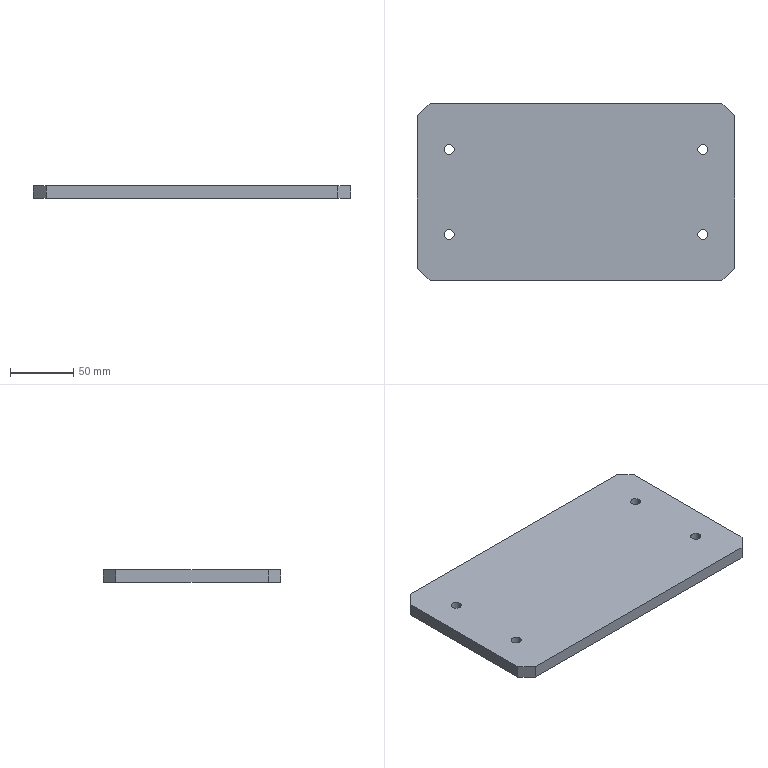Part | SolidWorks | features Cut 2, ICE 2, Extrusion 1 | 1 solid | 27 faces | box 250 x 140 x 10 mm | volume 345235 mm3 | cylinder 14 | plane 13 | commonest cylinder face diameters 8 x14
STEP:
#1=CARTESIAN_POINT('',(96.,-33.5,0.));
#2=VERTEX_POINT('',#1);
#3=CARTESIAN_POINT('',(104.,-33.5,0.));
#4=VERTEX_POINT('',#3);
#5=CARTESIAN_POINT('',(100.,-33.5,0.));
#6=DIRECTION('',(0.,0.,1.));
#7=DIRECTION('',(-1.,0.,0.));
#8=AXIS2_PLACEMENT_3D('',#5,#6,#7);
#9=CIRCLE('',#8,4.);
#10=EDGE_CURVE('',#2,#4,#9,.T.);
#11=ORIENTED_EDGE('',*,*,#10,.F.);
#12=CARTESIAN_POINT('',(96.,-33.5,10.));
#13=VERTEX_POINT('',#12);
#14=CARTESIAN_POINT('',(96.,-33.5,-11.314));
#15=DIRECTION('',(0.,0.,1.));
#16=VECTOR('',#15,1000.);
#17=LINE('',#14,#16);
#18=EDGE_CURVE('',#2,#13,#17,.T.);
#19=ORIENTED_EDGE('',*,*,#18,.T.);
#20=CARTESIAN_POINT('',(104.,-33.5,10.));
#21=VERTEX_POINT('',#20);
#22=CARTESIAN_POINT('',(100.,-33.5,10.));
#23=DIRECTION('',(0.,0.,1.));
#24=DIRECTION('',(-1.,0.,0.));
#25=AXIS2_PLACEMENT_3D('',#22,#23,#24);
#26=CIRCLE('',#25,4.);
#27=EDGE_CURVE('',#13,#21,#26,.T.);
#28=ORIENTED_EDGE('',*,*,#27,.T.);
#29=CARTESIAN_POINT('',(104.,-33.5,-11.314));
#30=DIRECTION('',(0.,0.,1.));
#31=VECTOR('',#30,1000.);
#32=LINE('',#29,#31);
#33=EDGE_CURVE('',#4,#21,#32,.T.);
#34=ORIENTED_EDGE('',*,*,#33,.F.);
#35=EDGE_LOOP('',(#11,#19,#28,#34));
#36=FACE_OUTER_BOUND('',#35,.T.);
#37=CARTESIAN_POINT('',(100.,-33.5,-11.314));
#38=DIRECTION('',(0.,0.,1.));
#39=DIRECTION('',(1.,0.,0.));
#40=AXIS2_PLACEMENT_3D('',#37,#38,#39);
#41=CYLINDRICAL_SURFACE('',#40,4.);
#42=ADVANCED_FACE('',(#36),#41,.F.);
#43=CARTESIAN_POINT('',(-104.,-33.5,0.));
#44=VERTEX_POINT('',#43);
#45=CARTESIAN_POINT('',(-96.,-33.5,0.));
#46=VERTEX_POINT('',#45);
#47=CARTESIAN_POINT('',(-100.,-33.5,0.));
#48=DIRECTION('',(0.,0.,1.));
#49=DIRECTION('',(-1.,0.,0.));
#50=AXIS2_PLACEMENT_3D('',#47,#48,#49);
#51=CIRCLE('',#50,4.);
#52=EDGE_CURVE('',#44,#46,#51,.T.);
#53=ORIENTED_EDGE('',*,*,#52,.F.);
#54=CARTESIAN_POINT('',(-104.,-33.5,10.));
#55=VERTEX_POINT('',#54);
#56=CARTESIAN_POINT('',(-104.,-33.5,-11.314));
#57=DIRECTION('',(0.,0.,1.));
#58=VECTOR('',#57,1000.);
#59=LINE('',#56,#58);
#60=EDGE_CURVE('',#44,#55,#59,.T.);
#61=ORIENTED_EDGE('',*,*,#60,.T.);
#62=CARTESIAN_POINT('',(-96.,-33.5,10.));
#63=VERTEX_POINT('',#62);
#64=CARTESIAN_POINT('',(-100.,-33.5,10.));
#65=DIRECTION('',(0.,0.,1.));
#66=DIRECTION('',(1.,0.,0.));
#67=AXIS2_PLACEMENT_3D('',#64,#65,#66);
#68=CIRCLE('',#67,4.);
#69=EDGE_CURVE('',#55,#63,#68,.T.);
#70=ORIENTED_EDGE('',*,*,#69,.T.);
#71=CARTESIAN_POINT('',(-96.,-33.5,-11.314));
#72=DIRECTION('',(0.,0.,1.));
#73=VECTOR('',#72,1000.);
#74=LINE('',#71,#73);
#75=EDGE_CURVE('',#46,#63,#74,.T.);
#76=ORIENTED_EDGE('',*,*,#75,.F.);
#77=EDGE_LOOP('',(#53,#61,#70,#76));
#78=FACE_OUTER_BOUND('',#77,.T.);
#79=CARTESIAN_POINT('',(-100.,-33.5,-11.314));
#80=DIRECTION('',(0.,0.,1.));
#81=DIRECTION('',(1.,0.,0.));
#82=AXIS2_PLACEMENT_3D('',#79,#80,#81);
#83=CYLINDRICAL_SURFACE('',#82,4.);
#84=ADVANCED_FACE('',(#78),#83,.F.);
#85=CARTESIAN_POINT('',(-104.,33.5,0.));
#86=VERTEX_POINT('',#85);
#87=CARTESIAN_POINT('',(-96.,33.5,0.));
#88=VERTEX_POINT('',#87);
#89=CARTESIAN_POINT('',(-100.,33.5,0.));
#90=DIRECTION('',(0.,0.,1.));
#91=DIRECTION('',(-1.,0.,0.));
#92=AXIS2_PLACEMENT_3D('',#89,#90,#91);
#93=CIRCLE('',#92,4.);
#94=EDGE_CURVE('',#86,#88,#93,.T.);
#95=ORIENTED_EDGE('',*,*,#94,.F.);
#96=CARTESIAN_POINT('',(-104.,33.5,10.));
#97=VERTEX_POINT('',#96);
#98=CARTESIAN_POINT('',(-104.,33.5,-11.314));
#99=DIRECTION('',(0.,0.,1.));
#100=VECTOR('',#99,1000.);
#101=LINE('',#98,#100);
#102=EDGE_CURVE('',#86,#97,#101,.T.);
#103=ORIENTED_EDGE('',*,*,#102,.T.);
#104=CARTESIAN_POINT('',(-96.,33.5,10.));
#105=VERTEX_POINT('',#104);
#106=CARTESIAN_POINT('',(-100.,33.5,10.));
#107=DIRECTION('',(0.,0.,1.));
#108=DIRECTION('',(-1.,0.,0.));
#109=AXIS2_PLACEMENT_3D('',#106,#107,#108);
#110=CIRCLE('',#109,4.);
#111=EDGE_CURVE('',#97,#105,#110,.T.);
#112=ORIENTED_EDGE('',*,*,#111,.T.);
#113=CARTESIAN_POINT('',(-96.,33.5,-11.314));
#114=DIRECTION('',(0.,0.,1.));
#115=VECTOR('',#114,1000.);
#116=LINE('',#113,#115);
#117=EDGE_CURVE('',#88,#105,#116,.T.);
#118=ORIENTED_EDGE('',*,*,#117,.F.);
#119=EDGE_LOOP('',(#95,#103,#112,#118));
#120=FACE_OUTER_BOUND('',#119,.T.);
#121=CARTESIAN_POINT('',(-100.,33.5,-11.314));
#122=DIRECTION('',(0.,0.,1.));
#123=DIRECTION('',(1.,0.,0.));
#124=AXIS2_PLACEMENT_3D('',#121,#122,#123);
#125=CYLINDRICAL_SURFACE('',#124,4.);
#126=ADVANCED_FACE('',(#120),#125,.F.);
#127=CARTESIAN_POINT('',(96.,33.5,0.));
#128=VERTEX_POINT('',#127);
#129=CARTESIAN_POINT('',(104.,33.5,0.));
#130=VERTEX_POINT('',#129);
#131=CARTESIAN_POINT('',(100.,33.5,0.));
#132=DIRECTION('',(0.,0.,1.));
#133=DIRECTION('',(-1.,0.,0.));
#134=AXIS2_PLACEMENT_3D('',#131,#132,#133);
#135=CIRCLE('',#134,4.);
#136=EDGE_CURVE('',#128,#130,#135,.T.);
#137=ORIENTED_EDGE('',*,*,#136,.F.);
#138=CARTESIAN_POINT('',(96.,33.5,10.));
#139=VERTEX_POINT('',#138);
#140=CARTESIAN_POINT('',(96.,33.5,-11.314));
#141=DIRECTION('',(0.,0.,1.));
#142=VECTOR('',#141,1000.);
#143=LINE('',#140,#142);
#144=EDGE_CURVE('',#128,#139,#143,.T.);
#145=ORIENTED_EDGE('',*,*,#144,.T.);
#146=CARTESIAN_POINT('',(104.,33.5,10.));
#147=VERTEX_POINT('',#146);
#148=CARTESIAN_POINT('',(100.,33.5,10.));
#149=DIRECTION('',(0.,0.,1.));
#150=DIRECTION('',(1.,0.,0.));
#151=AXIS2_PLACEMENT_3D('',#148,#149,#150);
#152=CIRCLE('',#151,4.);
#153=EDGE_CURVE('',#139,#147,#152,.T.);
#154=ORIENTED_EDGE('',*,*,#153,.T.);
#155=CARTESIAN_POINT('',(104.,33.5,-11.314));
#156=DIRECTION('',(0.,0.,1.));
#157=VECTOR('',#156,1000.);
#158=LINE('',#155,#157);
#159=EDGE_CURVE('',#130,#147,#158,.T.);
#160=ORIENTED_EDGE('',*,*,#159,.F.);
#161=EDGE_LOOP('',(#137,#145,#154,#160));
#162=FACE_OUTER_BOUND('',#161,.T.);
#163=CARTESIAN_POINT('',(100.,33.5,-11.314));
#164=DIRECTION('',(0.,0.,1.));
#165=DIRECTION('',(1.,0.,0.));
#166=AXIS2_PLACEMENT_3D('',#163,#164,#165);
#167=CYLINDRICAL_SURFACE('',#166,4.);
#168=ADVANCED_FACE('',(#162),#167,.F.);
#169=CARTESIAN_POINT('',(54.,-64.1,5.));
#170=VERTEX_POINT('',#169);
#171=CARTESIAN_POINT('',(46.,-64.1,5.));
#172=VERTEX_POINT('',#171);
#173=CARTESIAN_POINT('',(50.,-64.1,5.));
#174=DIRECTION('',(0.,0.,-1.));
#175=DIRECTION('',(-1.,0.,0.));
#176=AXIS2_PLACEMENT_3D('',#173,#174,#175);
#177=CIRCLE('',#176,4.);
#178=EDGE_CURVE('',#170,#172,#177,.T.);
#179=ORIENTED_EDGE('',*,*,#178,.F.);
#180=CARTESIAN_POINT('',(54.,-64.1,0.));
#181=VERTEX_POINT('',#180);
#182=CARTESIAN_POINT('',(54.,-64.1,5.));
#183=DIRECTION('',(0.,0.,-1.));
#184=VECTOR('',#183,1000.);
#185=LINE('',#182,#184);
#186=EDGE_CURVE('',#170,#181,#185,.T.);
#187=ORIENTED_EDGE('',*,*,#186,.T.);
#188=CARTESIAN_POINT('',(46.,-64.1,0.));
#189=VERTEX_POINT('',#188);
#190=CARTESIAN_POINT('',(50.,-64.1,0.));
#191=DIRECTION('',(0.,0.,-1.));
#192=DIRECTION('',(-1.,0.,0.));
#193=AXIS2_PLACEMENT_3D('',#190,#191,#192);
#194=CIRCLE('',#193,4.);
#195=EDGE_CURVE('',#181,#189,#194,.T.);
#196=ORIENTED_EDGE('',*,*,#195,.T.);
#197=CARTESIAN_POINT('',(46.,-64.1,5.));
#198=DIRECTION('',(0.,0.,-1.));
#199=VECTOR('',#198,1000.);
#200=LINE('',#197,#199);
#201=EDGE_CURVE('',#172,#189,#200,.T.);
#202=ORIENTED_EDGE('',*,*,#201,.F.);
#203=EDGE_LOOP('',(#179,#187,#196,#202));
#204=FACE_OUTER_BOUND('',#203,.T.);
#205=CARTESIAN_POINT('',(50.,-64.1,5.));
#206=DIRECTION('',(0.,0.,-1.));
#207=DIRECTION('',(-1.,0.,0.));
#208=AXIS2_PLACEMENT_3D('',#205,#206,#207);
#209=CYLINDRICAL_SURFACE('',#208,4.);
#210=ADVANCED_FACE('',(#204),#209,.F.);
#211=CARTESIAN_POINT('',(-46.,-64.1,5.));
#212=VERTEX_POINT('',#211);
#213=CARTESIAN_POINT('',(-54.,-64.1,5.));
#214=VERTEX_POINT('',#213);
#215=CARTESIAN_POINT('',(-50.,-64.1,5.));
#216=DIRECTION('',(0.,0.,-1.));
#217=DIRECTION('',(1.,0.,0.));
#218=AXIS2_PLACEMENT_3D('',#215,#216,#217);
#219=CIRCLE('',#218,4.);
#220=EDGE_CURVE('',#212,#214,#219,.T.);
#221=ORIENTED_EDGE('',*,*,#220,.F.);
#222=CARTESIAN_POINT('',(-46.,-64.1,0.));
#223=VERTEX_POINT('',#222);
#224=CARTESIAN_POINT('',(-46.,-64.1,5.));
#225=DIRECTION('',(0.,0.,-1.));
#226=VECTOR('',#225,1000.);
#227=LINE('',#224,#226);
#228=EDGE_CURVE('',#212,#223,#227,.T.);
#229=ORIENTED_EDGE('',*,*,#228,.T.);
#230=CARTESIAN_POINT('',(-54.,-64.1,0.));
#231=VERTEX_POINT('',#230);
#232=CARTESIAN_POINT('',(-50.,-64.1,0.));
#233=DIRECTION('',(0.,0.,-1.));
#234=DIRECTION('',(1.,0.,0.));
#235=AXIS2_PLACEMENT_3D('',#232,#233,#234);
#236=CIRCLE('',#235,4.);
#237=EDGE_CURVE('',#223,#231,#236,.T.);
#238=ORIENTED_EDGE('',*,*,#237,.T.);
#239=CARTESIAN_POINT('',(-54.,-64.1,5.));
#240=DIRECTION('',(0.,0.,-1.));
#241=VECTOR('',#240,1000.);
#242=LINE('',#239,#241);
#243=EDGE_CURVE('',#214,#231,#242,.T.);
#244=ORIENTED_EDGE('',*,*,#243,.F.);
#245=EDGE_LOOP('',(#221,#229,#238,#244));
#246=FACE_OUTER_BOUND('',#245,.T.);
#247=CARTESIAN_POINT('',(-50.,-64.1,5.));
#248=DIRECTION('',(0.,0.,-1.));
#249=DIRECTION('',(-1.,0.,0.));
#250=AXIS2_PLACEMENT_3D('',#247,#248,#249);
#251=CYLINDRICAL_SURFACE('',#250,4.);
#252=ADVANCED_FACE('',(#246),#251,.F.);
#253=CARTESIAN_POINT('',(83.1,0.,5.));
#254=VERTEX_POINT('',#253);
#255=CARTESIAN_POINT('',(75.1,0.,5.));
#256=VERTEX_POINT('',#255);
#257=CARTESIAN_POINT('',(79.1,0.,5.));
#258=DIRECTION('',(0.,0.,-1.));
#259=DIRECTION('',(1.,0.,0.));
#260=AXIS2_PLACEMENT_3D('',#257,#258,#259);
#261=CIRCLE('',#260,4.);
#262=EDGE_CURVE('',#254,#256,#261,.T.);
#263=ORIENTED_EDGE('',*,*,#262,.F.);
#264=CARTESIAN_POINT('',(83.1,0.,0.));
#265=VERTEX_POINT('',#264);
#266=CARTESIAN_POINT('',(83.1,0.,5.));
#267=DIRECTION('',(0.,0.,-1.));
#268=VECTOR('',#267,1000.);
#269=LINE('',#266,#268);
#270=EDGE_CURVE('',#254,#265,#269,.T.);
#271=ORIENTED_EDGE('',*,*,#270,.T.);
#272=CARTESIAN_POINT('',(75.1,0.,0.));
#273=VERTEX_POINT('',#272);
#274=CARTESIAN_POINT('',(79.1,0.,0.));
#275=DIRECTION('',(0.,0.,-1.));
#276=DIRECTION('',(1.,0.,0.));
#277=AXIS2_PLACEMENT_3D('',#274,#275,#276);
#278=CIRCLE('',#277,4.);
#279=EDGE_CURVE('',#265,#273,#278,.T.);
#280=ORIENTED_EDGE('',*,*,#279,.T.);
#281=CARTESIAN_POINT('',(75.1,0.,5.));
#282=DIRECTION('',(0.,0.,-1.));
#283=VECTOR('',#282,1000.);
#284=LINE('',#281,#283);
#285=EDGE_CURVE('',#256,#273,#284,.T.);
#286=ORIENTED_EDGE('',*,*,#285,.F.);
#287=EDGE_LOOP('',(#263,#271,#280,#286));
#288=FACE_OUTER_BOUND('',#287,.T.);
#289=CARTESIAN_POINT('',(79.1,0.,5.));
#290=DIRECTION('',(0.,0.,-1.));
#291=DIRECTION('',(-1.,0.,0.));
#292=AXIS2_PLACEMENT_3D('',#289,#290,#291);
#293=CYLINDRICAL_SURFACE('',#292,4.);
#294=ADVANCED_FACE('',(#288),#293,.F.);
#295=CARTESIAN_POINT('',(115.,70.,0.));
#296=VERTEX_POINT('',#295);
#297=CARTESIAN_POINT('',(-115.,70.,0.));
#298=VERTEX_POINT('',#297);
#299=CARTESIAN_POINT('',(115.,70.,0.));
#300=DIRECTION('',(-1.,0.,0.));
#301=VECTOR('',#300,1000.);
#302=LINE('',#299,#301);
#303=EDGE_CURVE('',#296,#298,#302,.T.);
#304=ORIENTED_EDGE('',*,*,#303,.T.);
#305=CARTESIAN_POINT('',(-115.,70.,10.));
#306=VERTEX_POINT('',#305);
#307=CARTESIAN_POINT('',(-115.,70.,10.));
#308=DIRECTION('',(0.,0.,-1.));
#309=VECTOR('',#308,1000.);
#310=LINE('',#307,#309);
#311=EDGE_CURVE('',#306,#298,#310,.T.);
#312=ORIENTED_EDGE('',*,*,#311,.F.);
#313=CARTESIAN_POINT('',(115.,70.,10.));
#314=VERTEX_POINT('',#313);
#315=CARTESIAN_POINT('',(115.,70.,10.));
#316=DIRECTION('',(-1.,0.,0.));
#317=VECTOR('',#316,1000.);
#318=LINE('',#315,#317);
#319=EDGE_CURVE('',#314,#306,#318,.T.);
#320=ORIENTED_EDGE('',*,*,#319,.F.);
#321=CARTESIAN_POINT('',(115.,70.,10.));
#322=DIRECTION('',(0.,0.,-1.));
#323=VECTOR('',#322,1000.);
#324=LINE('',#321,#323);
#325=EDGE_CURVE('',#314,#296,#324,.T.);
#326=ORIENTED_EDGE('',*,*,#325,.T.);
#327=EDGE_LOOP('',(#304,#312,#320,#326));
#328=FACE_OUTER_BOUND('',#327,.T.);
#329=CARTESIAN_POINT('',(115.,70.,10.));
#330=DIRECTION('',(0.,-1.,0.));
#331=DIRECTION('',(1.,0.,0.));
#332=AXIS2_PLACEMENT_3D('',#329,#330,#331);
#333=PLANE('',#332);
#334=ADVANCED_FACE('',(#328),#333,.F.);
#335=CARTESIAN_POINT('',(-125.,60.,0.));
#336=VERTEX_POINT('',#335);
#337=CARTESIAN_POINT('',(-115.,70.,0.));
#338=DIRECTION('',(-0.7071,-0.7071,0.));
#339=VECTOR('',#338,1000.);
#340=LINE('',#337,#339);
#341=EDGE_CURVE('',#298,#336,#340,.T.);
#342=ORIENTED_EDGE('',*,*,#341,.T.);
#343=CARTESIAN_POINT('',(-125.,60.,10.));
#344=VERTEX_POINT('',#343);
#345=CARTESIAN_POINT('',(-125.,60.,10.));
#346=DIRECTION('',(0.,0.,-1.));
#347=VECTOR('',#346,1000.);
#348=LINE('',#345,#347);
#349=EDGE_CURVE('',#344,#336,#348,.T.);
#350=ORIENTED_EDGE('',*,*,#349,.F.);
#351=CARTESIAN_POINT('',(-115.,70.,10.));
#352=DIRECTION('',(-0.7071,-0.7071,0.));
#353=VECTOR('',#352,1000.);
#354=LINE('',#351,#353);
#355=EDGE_CURVE('',#306,#344,#354,.T.);
#356=ORIENTED_EDGE('',*,*,#355,.F.);
#357=ORIENTED_EDGE('',*,*,#311,.T.);
#358=EDGE_LOOP('',(#342,#350,#356,#357));
#359=FACE_OUTER_BOUND('',#358,.T.);
#360=CARTESIAN_POINT('',(-115.,70.,10.));
#361=DIRECTION('',(0.7071,-0.7071,0.));
#362=DIRECTION('',(0.7071,0.7071,0.));
#363=AXIS2_PLACEMENT_3D('',#360,#361,#362);
#364=PLANE('',#363);
#365=ADVANCED_FACE('',(#359),#364,.F.);
#366=CARTESIAN_POINT('',(-125.,-60.,0.));
#367=VERTEX_POINT('',#366);
#368=CARTESIAN_POINT('',(-125.,-60.,0.));
#369=DIRECTION('',(0.,-1.,0.));
#370=VECTOR('',#369,1000.);
#371=LINE('',#368,#370);
#372=EDGE_CURVE('',#336,#367,#371,.T.);
#373=ORIENTED_EDGE('',*,*,#372,.T.);
#374=CARTESIAN_POINT('',(-125.,-60.,10.));
#375=VERTEX_POINT('',#374);
#376=CARTESIAN_POINT('',(-125.,-60.,10.));
#377=DIRECTION('',(0.,0.,-1.));
#378=VECTOR('',#377,1000.);
#379=LINE('',#376,#378);
#380=EDGE_CURVE('',#375,#367,#379,.T.);
#381=ORIENTED_EDGE('',*,*,#380,.F.);
#382=CARTESIAN_POINT('',(-125.,-60.,10.));
#383=DIRECTION('',(0.,-1.,0.));
#384=VECTOR('',#383,1000.);
#385=LINE('',#382,#384);
#386=EDGE_CURVE('',#344,#375,#385,.T.);
#387=ORIENTED_EDGE('',*,*,#386,.F.);
#388=ORIENTED_EDGE('',*,*,#349,.T.);
#389=EDGE_LOOP('',(#373,#381,#387,#388));
#390=FACE_OUTER_BOUND('',#389,.T.);
#391=CARTESIAN_POINT('',(-125.,-60.,10.));
#392=DIRECTION('',(1.,0.,0.));
#393=DIRECTION('',(0.,0.,-1.));
#394=AXIS2_PLACEMENT_3D('',#391,#392,#393);
#395=PLANE('',#394);
#396=ADVANCED_FACE('',(#390),#395,.F.);
#397=CARTESIAN_POINT('',(-115.,-70.,0.));
#398=VERTEX_POINT('',#397);
#399=CARTESIAN_POINT('',(-115.,-70.,0.));
#400=DIRECTION('',(0.7071,-0.7071,0.));
#401=VECTOR('',#400,1000.);
#402=LINE('',#399,#401);
#403=EDGE_CURVE('',#367,#398,#402,.T.);
#404=ORIENTED_EDGE('',*,*,#403,.T.);
#405=CARTESIAN_POINT('',(-115.,-70.,10.));
#406=VERTEX_POINT('',#405);
#407=CARTESIAN_POINT('',(-115.,-70.,10.));
#408=DIRECTION('',(0.,0.,-1.));
#409=VECTOR('',#408,1000.);
#410=LINE('',#407,#409);
#411=EDGE_CURVE('',#406,#398,#410,.T.);
#412=ORIENTED_EDGE('',*,*,#411,.F.);
#413=CARTESIAN_POINT('',(-115.,-70.,10.));
#414=DIRECTION('',(0.7071,-0.7071,0.));
#415=VECTOR('',#414,1000.);
#416=LINE('',#413,#415);
#417=EDGE_CURVE('',#375,#406,#416,.T.);
#418=ORIENTED_EDGE('',*,*,#417,.F.);
#419=ORIENTED_EDGE('',*,*,#380,.T.);
#420=EDGE_LOOP('',(#404,#412,#418,#419));
#421=FACE_OUTER_BOUND('',#420,.T.);
#422=CARTESIAN_POINT('',(-115.,-70.,10.));
#423=DIRECTION('',(0.7071,0.7071,0.));
#424=DIRECTION('',(-0.7071,0.7071,0.));
#425=AXIS2_PLACEMENT_3D('',#422,#423,#424);
#426=PLANE('',#425);
#427=ADVANCED_FACE('',(#421),#426,.F.);
#428=CARTESIAN_POINT('',(115.,-70.,0.));
#429=VERTEX_POINT('',#428);
#430=CARTESIAN_POINT('',(115.,-70.,0.));
#431=DIRECTION('',(1.,0.,0.));
#432=VECTOR('',#431,1000.);
#433=LINE('',#430,#432);
#434=EDGE_CURVE('',#398,#429,#433,.T.);
#435=ORIENTED_EDGE('',*,*,#434,.T.);
#436=CARTESIAN_POINT('',(115.,-70.,10.));
#437=VERTEX_POINT('',#436);
#438=CARTESIAN_POINT('',(115.,-70.,10.));
#439=DIRECTION('',(0.,0.,-1.));
#440=VECTOR('',#439,1000.);
#441=LINE('',#438,#440);
#442=EDGE_CURVE('',#437,#429,#441,.T.);
#443=ORIENTED_EDGE('',*,*,#442,.F.);
#444=CARTESIAN_POINT('',(115.,-70.,10.));
#445=DIRECTION('',(1.,0.,0.));
#446=VECTOR('',#445,1000.);
#447=LINE('',#444,#446);
#448=EDGE_CURVE('',#406,#437,#447,.T.);
#449=ORIENTED_EDGE('',*,*,#448,.F.);
#450=ORIENTED_EDGE('',*,*,#411,.T.);
#451=EDGE_LOOP('',(#435,#443,#449,#450));
#452=FACE_OUTER_BOUND('',#451,.T.);
#453=CARTESIAN_POINT('',(115.,-70.,10.));
#454=DIRECTION('',(0.,1.,0.));
#455=DIRECTION('',(-1.,0.,0.));
#456=AXIS2_PLACEMENT_3D('',#453,#454,#455);
#457=PLANE('',#456);
#458=ADVANCED_FACE('',(#452),#457,.F.);
#459=CARTESIAN_POINT('',(125.,-60.,0.));
#460=VERTEX_POINT('',#459);
#461=CARTESIAN_POINT('',(115.,-70.,0.));
#462=DIRECTION('',(0.7071,0.7071,0.));
#463=VECTOR('',#462,1000.);
#464=LINE('',#461,#463);
#465=EDGE_CURVE('',#429,#460,#464,.T.);
#466=ORIENTED_EDGE('',*,*,#465,.T.);
#467=CARTESIAN_POINT('',(125.,-60.,10.));
#468=VERTEX_POINT('',#467);
#469=CARTESIAN_POINT('',(125.,-60.,10.));
#470=DIRECTION('',(0.,0.,-1.));
#471=VECTOR('',#470,1000.);
#472=LINE('',#469,#471);
#473=EDGE_CURVE('',#468,#460,#472,.T.);
#474=ORIENTED_EDGE('',*,*,#473,.F.);
#475=CARTESIAN_POINT('',(115.,-70.,10.));
#476=DIRECTION('',(0.7071,0.7071,0.));
#477=VECTOR('',#476,1000.);
#478=LINE('',#475,#477);
#479=EDGE_CURVE('',#437,#468,#478,.T.);
#480=ORIENTED_EDGE('',*,*,#479,.F.);
#481=ORIENTED_EDGE('',*,*,#442,.T.);
#482=EDGE_LOOP('',(#466,#474,#480,#481));
#483=FACE_OUTER_BOUND('',#482,.T.);
#484=CARTESIAN_POINT('',(115.,-70.,10.));
#485=DIRECTION('',(-0.7071,0.7071,0.));
#486=DIRECTION('',(-0.7071,-0.7071,0.));
#487=AXIS2_PLACEMENT_3D('',#484,#485,#486);
#488=PLANE('',#487);
#489=ADVANCED_FACE('',(#483),#488,.F.);
#490=CARTESIAN_POINT('',(125.,60.,0.));
#491=VERTEX_POINT('',#490);
#492=CARTESIAN_POINT('',(125.,-60.,0.));
#493=DIRECTION('',(0.,1.,0.));
#494=VECTOR('',#493,1000.);
#495=LINE('',#492,#494);
#496=EDGE_CURVE('',#460,#491,#495,.T.);
#497=ORIENTED_EDGE('',*,*,#496,.T.);
#498=CARTESIAN_POINT('',(125.,60.,10.));
#499=VERTEX_POINT('',#498);
#500=CARTESIAN_POINT('',(125.,60.,10.));
#501=DIRECTION('',(0.,0.,-1.));
#502=VECTOR('',#501,1000.);
#503=LINE('',#500,#502);
#504=EDGE_CURVE('',#499,#491,#503,.T.);
#505=ORIENTED_EDGE('',*,*,#504,.F.);
#506=CARTESIAN_POINT('',(125.,-60.,10.));
#507=DIRECTION('',(0.,1.,0.));
#508=VECTOR('',#507,1000.);
#509=LINE('',#506,#508);
#510=EDGE_CURVE('',#468,#499,#509,.T.);
#511=ORIENTED_EDGE('',*,*,#510,.F.);
#512=ORIENTED_EDGE('',*,*,#473,.T.);
#513=EDGE_LOOP('',(#497,#505,#511,#512));
#514=FACE_OUTER_BOUND('',#513,.T.);
#515=CARTESIAN_POINT('',(125.,-60.,10.));
#516=DIRECTION('',(-1.,0.,0.));
#517=DIRECTION('',(0.,0.,1.));
#518=AXIS2_PLACEMENT_3D('',#515,#516,#517);
#519=PLANE('',#518);
#520=ADVANCED_FACE('',(#514),#519,.F.);
#521=CARTESIAN_POINT('',(125.,60.,0.));
#522=DIRECTION('',(-0.7071,0.7071,0.));
#523=VECTOR('',#522,1000.);
#524=LINE('',#521,#523);
#525=EDGE_CURVE('',#491,#296,#524,.T.);
#526=ORIENTED_EDGE('',*,*,#525,.T.);
#527=ORIENTED_EDGE('',*,*,#325,.F.);
#528=CARTESIAN_POINT('',(125.,60.,10.));
#529=DIRECTION('',(-0.7071,0.7071,0.));
#530=VECTOR('',#529,1000.);
#531=LINE('',#528,#530);
#532=EDGE_CURVE('',#499,#314,#531,.T.);
#533=ORIENTED_EDGE('',*,*,#532,.F.);
#534=ORIENTED_EDGE('',*,*,#504,.T.);
#535=EDGE_LOOP('',(#526,#527,#533,#534));
#536=FACE_OUTER_BOUND('',#535,.T.);
#537=CARTESIAN_POINT('',(125.,60.,10.));
#538=DIRECTION('',(-0.7071,-0.7071,0.));
#539=DIRECTION('',(0.7071,-0.7071,0.));
#540=AXIS2_PLACEMENT_3D('',#537,#538,#539);
#541=PLANE('',#540);
#542=ADVANCED_FACE('',(#536),#541,.F.);
#543=CARTESIAN_POINT('',(100.,-33.5,10.));
#544=DIRECTION('',(0.,0.,1.));
#545=DIRECTION('',(-1.,0.,0.));
#546=AXIS2_PLACEMENT_3D('',#543,#544,#545);
#547=CIRCLE('',#546,4.);
#548=EDGE_CURVE('',#21,#13,#547,.T.);
#549=ORIENTED_EDGE('',*,*,#548,.F.);
#550=ORIENTED_EDGE('',*,*,#27,.F.);
#551=EDGE_LOOP('',(#549,#550));
#552=FACE_BOUND('',#551,.T.);
#553=CARTESIAN_POINT('',(-100.,-33.5,10.));
#554=DIRECTION('',(0.,0.,1.));
#555=DIRECTION('',(1.,0.,0.));
#556=AXIS2_PLACEMENT_3D('',#553,#554,#555);
#557=CIRCLE('',#556,4.);
#558=EDGE_CURVE('',#63,#55,#557,.T.);
#559=ORIENTED_EDGE('',*,*,#558,.F.);
#560=ORIENTED_EDGE('',*,*,#69,.F.);
#561=EDGE_LOOP('',(#559,#560));
#562=FACE_BOUND('',#561,.T.);
#563=CARTESIAN_POINT('',(-100.,33.5,10.));
#564=DIRECTION('',(0.,0.,1.));
#565=DIRECTION('',(-1.,0.,0.));
#566=AXIS2_PLACEMENT_3D('',#563,#564,#565);
#567=CIRCLE('',#566,4.);
#568=EDGE_CURVE('',#105,#97,#567,.T.);
#569=ORIENTED_EDGE('',*,*,#568,.F.);
#570=ORIENTED_EDGE('',*,*,#111,.F.);
#571=EDGE_LOOP('',(#569,#570));
#572=FACE_BOUND('',#571,.T.);
#573=CARTESIAN_POINT('',(100.,33.5,10.));
#574=DIRECTION('',(0.,0.,1.));
#575=DIRECTION('',(1.,0.,0.));
#576=AXIS2_PLACEMENT_3D('',#573,#574,#575);
#577=CIRCLE('',#576,4.);
#578=EDGE_CURVE('',#147,#139,#577,.T.);
#579=ORIENTED_EDGE('',*,*,#578,.F.);
#580=ORIENTED_EDGE('',*,*,#153,.F.);
#581=EDGE_LOOP('',(#579,#580));
#582=FACE_BOUND('',#581,.T.);
#583=ORIENTED_EDGE('',*,*,#319,.T.);
#584=ORIENTED_EDGE('',*,*,#355,.T.);
#585=ORIENTED_EDGE('',*,*,#386,.T.);
#586=ORIENTED_EDGE('',*,*,#417,.T.);
#587=ORIENTED_EDGE('',*,*,#448,.T.);
#588=ORIENTED_EDGE('',*,*,#479,.T.);
#589=ORIENTED_EDGE('',*,*,#510,.T.);
#590=ORIENTED_EDGE('',*,*,#532,.T.);
#591=EDGE_LOOP('',(#583,#584,#585,#586,#587,#588,#589,#590));
#592=FACE_OUTER_BOUND('',#591,.T.);
#593=CARTESIAN_POINT('',(0.,0.,10.));
#594=DIRECTION('',(0.,0.,-1.));
#595=DIRECTION('',(-1.,0.,0.));
#596=AXIS2_PLACEMENT_3D('',#593,#594,#595);
#597=PLANE('',#596);
#598=ADVANCED_FACE('',(#552,#562,#572,#582,#592),#597,.F.);
#599=CARTESIAN_POINT('',(100.,-33.5,0.));
#600=DIRECTION('',(0.,0.,1.));
#601=DIRECTION('',(-1.,0.,0.));
#602=AXIS2_PLACEMENT_3D('',#599,#600,#601);
#603=CIRCLE('',#602,4.);
#604=EDGE_CURVE('',#4,#2,#603,.T.);
#605=ORIENTED_EDGE('',*,*,#604,.T.);
#606=ORIENTED_EDGE('',*,*,#10,.T.);
#607=EDGE_LOOP('',(#605,#606));
#608=FACE_BOUND('',#607,.T.);
#609=CARTESIAN_POINT('',(-100.,-33.5,0.));
#610=DIRECTION('',(0.,0.,1.));
#611=DIRECTION('',(-1.,0.,0.));
#612=AXIS2_PLACEMENT_3D('',#609,#610,#611);
#613=CIRCLE('',#612,4.);
#614=EDGE_CURVE('',#46,#44,#613,.T.);
#615=ORIENTED_EDGE('',*,*,#614,.T.);
#616=ORIENTED_EDGE('',*,*,#52,.T.);
#617=EDGE_LOOP('',(#615,#616));
#618=FACE_BOUND('',#617,.T.);
#619=CARTESIAN_POINT('',(-100.,33.5,0.));
#620=DIRECTION('',(0.,0.,1.));
#621=DIRECTION('',(-1.,0.,0.));
#622=AXIS2_PLACEMENT_3D('',#619,#620,#621);
#623=CIRCLE('',#622,4.);
#624=EDGE_CURVE('',#88,#86,#623,.T.);
#625=ORIENTED_EDGE('',*,*,#624,.T.);
#626=ORIENTED_EDGE('',*,*,#94,.T.);
#627=EDGE_LOOP('',(#625,#626));
#628=FACE_BOUND('',#627,.T.);
#629=CARTESIAN_POINT('',(100.,33.5,0.));
#630=DIRECTION('',(0.,0.,1.));
#631=DIRECTION('',(-1.,0.,0.));
#632=AXIS2_PLACEMENT_3D('',#629,#630,#631);
#633=CIRCLE('',#632,4.);
#634=EDGE_CURVE('',#130,#128,#633,.T.);
#635=ORIENTED_EDGE('',*,*,#634,.T.);
#636=ORIENTED_EDGE('',*,*,#136,.T.);
#637=EDGE_LOOP('',(#635,#636));
#638=FACE_BOUND('',#637,.T.);
#639=CARTESIAN_POINT('',(50.,-64.1,0.));
#640=DIRECTION('',(0.,0.,-1.));
#641=DIRECTION('',(-1.,0.,0.));
#642=AXIS2_PLACEMENT_3D('',#639,#640,#641);
#643=CIRCLE('',#642,4.);
#644=EDGE_CURVE('',#189,#181,#643,.T.);
#645=ORIENTED_EDGE('',*,*,#644,.F.);
#646=ORIENTED_EDGE('',*,*,#195,.F.);
#647=EDGE_LOOP('',(#645,#646));
#648=FACE_BOUND('',#647,.T.);
#649=CARTESIAN_POINT('',(-50.,-64.1,0.));
#650=DIRECTION('',(0.,0.,-1.));
#651=DIRECTION('',(1.,0.,0.));
#652=AXIS2_PLACEMENT_3D('',#649,#650,#651);
#653=CIRCLE('',#652,4.);
#654=EDGE_CURVE('',#231,#223,#653,.T.);
#655=ORIENTED_EDGE('',*,*,#654,.F.);
#656=ORIENTED_EDGE('',*,*,#237,.F.);
#657=EDGE_LOOP('',(#655,#656));
#658=FACE_BOUND('',#657,.T.);
#659=CARTESIAN_POINT('',(79.1,0.,0.));
#660=DIRECTION('',(0.,0.,-1.));
#661=DIRECTION('',(1.,0.,0.));
#662=AXIS2_PLACEMENT_3D('',#659,#660,#661);
#663=CIRCLE('',#662,4.);
#664=EDGE_CURVE('',#273,#265,#663,.T.);
#665=ORIENTED_EDGE('',*,*,#664,.F.);
#666=ORIENTED_EDGE('',*,*,#279,.F.);
#667=EDGE_LOOP('',(#665,#666));
#668=FACE_BOUND('',#667,.T.);
#669=ORIENTED_EDGE('',*,*,#303,.F.);
#670=ORIENTED_EDGE('',*,*,#525,.F.);
#671=ORIENTED_EDGE('',*,*,#496,.F.);
#672=ORIENTED_EDGE('',*,*,#465,.F.);
#673=ORIENTED_EDGE('',*,*,#434,.F.);
#674=ORIENTED_EDGE('',*,*,#403,.F.);
#675=ORIENTED_EDGE('',*,*,#372,.F.);
#676=ORIENTED_EDGE('',*,*,#341,.F.);
#677=EDGE_LOOP('',(#669,#670,#671,#672,#673,#674,#675,#676));
#678=FACE_OUTER_BOUND('',#677,.T.);
#679=CARTESIAN_POINT('',(0.,0.,0.));
#680=DIRECTION('',(0.,0.,-1.));
#681=DIRECTION('',(-1.,0.,0.));
#682=AXIS2_PLACEMENT_3D('',#679,#680,#681);
#683=PLANE('',#682);
#684=ADVANCED_FACE('',(#608,#618,#628,#638,#648,#658,#668,#678),#683,.T.);
#685=ORIENTED_EDGE('',*,*,#270,.F.);
#686=CARTESIAN_POINT('',(79.1,0.,5.));
#687=DIRECTION('',(0.,0.,-1.));
#688=DIRECTION('',(1.,0.,0.));
#689=AXIS2_PLACEMENT_3D('',#686,#687,#688);
#690=CIRCLE('',#689,4.);
#691=EDGE_CURVE('',#256,#254,#690,.T.);
#692=ORIENTED_EDGE('',*,*,#691,.F.);
#693=ORIENTED_EDGE('',*,*,#285,.T.);
#694=ORIENTED_EDGE('',*,*,#664,.T.);
#695=EDGE_LOOP('',(#685,#692,#693,#694));
#696=FACE_OUTER_BOUND('',#695,.T.);
#697=CARTESIAN_POINT('',(79.1,0.,5.));
#698=DIRECTION('',(0.,0.,-1.));
#699=DIRECTION('',(-1.,0.,0.));
#700=AXIS2_PLACEMENT_3D('',#697,#698,#699);
#701=CYLINDRICAL_SURFACE('',#700,4.);
#702=ADVANCED_FACE('',(#696),#701,.F.);
#703=ORIENTED_EDGE('',*,*,#691,.T.);
#704=ORIENTED_EDGE('',*,*,#262,.T.);
#705=EDGE_LOOP('',(#703,#704));
#706=FACE_OUTER_BOUND('',#705,.T.);
#707=CARTESIAN_POINT('',(79.1,0.,5.));
#708=DIRECTION('',(0.,0.,1.));
#709=DIRECTION('',(1.,0.,0.));
#710=AXIS2_PLACEMENT_3D('',#707,#708,#709);
#711=PLANE('',#710);
#712=ADVANCED_FACE('',(#706),#711,.F.);
#713=ORIENTED_EDGE('',*,*,#228,.F.);
#714=CARTESIAN_POINT('',(-50.,-64.1,5.));
#715=DIRECTION('',(0.,0.,-1.));
#716=DIRECTION('',(1.,0.,0.));
#717=AXIS2_PLACEMENT_3D('',#714,#715,#716);
#718=CIRCLE('',#717,4.);
#719=EDGE_CURVE('',#214,#212,#718,.T.);
#720=ORIENTED_EDGE('',*,*,#719,.F.);
#721=ORIENTED_EDGE('',*,*,#243,.T.);
#722=ORIENTED_EDGE('',*,*,#654,.T.);
#723=EDGE_LOOP('',(#713,#720,#721,#722));
#724=FACE_OUTER_BOUND('',#723,.T.);
#725=CARTESIAN_POINT('',(-50.,-64.1,5.));
#726=DIRECTION('',(0.,0.,-1.));
#727=DIRECTION('',(-1.,0.,0.));
#728=AXIS2_PLACEMENT_3D('',#725,#726,#727);
#729=CYLINDRICAL_SURFACE('',#728,4.);
#730=ADVANCED_FACE('',(#724),#729,.F.);
#731=ORIENTED_EDGE('',*,*,#719,.T.);
#732=ORIENTED_EDGE('',*,*,#220,.T.);
#733=EDGE_LOOP('',(#731,#732));
#734=FACE_OUTER_BOUND('',#733,.T.);
#735=CARTESIAN_POINT('',(-50.,-64.1,5.));
#736=DIRECTION('',(0.,0.,1.));
#737=DIRECTION('',(1.,0.,0.));
#738=AXIS2_PLACEMENT_3D('',#735,#736,#737);
#739=PLANE('',#738);
#740=ADVANCED_FACE('',(#734),#739,.F.);
#741=ORIENTED_EDGE('',*,*,#186,.F.);
#742=CARTESIAN_POINT('',(50.,-64.1,5.));
#743=DIRECTION('',(0.,0.,-1.));
#744=DIRECTION('',(-1.,0.,0.));
#745=AXIS2_PLACEMENT_3D('',#742,#743,#744);
#746=CIRCLE('',#745,4.);
#747=EDGE_CURVE('',#172,#170,#746,.T.);
#748=ORIENTED_EDGE('',*,*,#747,.F.);
#749=ORIENTED_EDGE('',*,*,#201,.T.);
#750=ORIENTED_EDGE('',*,*,#644,.T.);
#751=EDGE_LOOP('',(#741,#748,#749,#750));
#752=FACE_OUTER_BOUND('',#751,.T.);
#753=CARTESIAN_POINT('',(50.,-64.1,5.));
#754=DIRECTION('',(0.,0.,-1.));
#755=DIRECTION('',(-1.,0.,0.));
#756=AXIS2_PLACEMENT_3D('',#753,#754,#755);
#757=CYLINDRICAL_SURFACE('',#756,4.);
#758=ADVANCED_FACE('',(#752),#757,.F.);
#759=ORIENTED_EDGE('',*,*,#747,.T.);
#760=ORIENTED_EDGE('',*,*,#178,.T.);
#761=EDGE_LOOP('',(#759,#760));
#762=FACE_OUTER_BOUND('',#761,.T.);
#763=CARTESIAN_POINT('',(50.,-64.1,5.));
#764=DIRECTION('',(0.,0.,-1.));
#765=DIRECTION('',(-1.,0.,0.));
#766=AXIS2_PLACEMENT_3D('',#763,#764,#765);
#767=PLANE('',#766);
#768=ADVANCED_FACE('',(#762),#767,.T.);
#769=ORIENTED_EDGE('',*,*,#144,.F.);
#770=ORIENTED_EDGE('',*,*,#634,.F.);
#771=ORIENTED_EDGE('',*,*,#159,.T.);
#772=ORIENTED_EDGE('',*,*,#578,.T.);
#773=EDGE_LOOP('',(#769,#770,#771,#772));
#774=FACE_OUTER_BOUND('',#773,.T.);
#775=CARTESIAN_POINT('',(100.,33.5,-11.314));
#776=DIRECTION('',(0.,0.,1.));
#777=DIRECTION('',(1.,0.,0.));
#778=AXIS2_PLACEMENT_3D('',#775,#776,#777);
#779=CYLINDRICAL_SURFACE('',#778,4.);
#780=ADVANCED_FACE('',(#774),#779,.F.);
#781=ORIENTED_EDGE('',*,*,#102,.F.);
#782=ORIENTED_EDGE('',*,*,#624,.F.);
#783=ORIENTED_EDGE('',*,*,#117,.T.);
#784=ORIENTED_EDGE('',*,*,#568,.T.);
#785=EDGE_LOOP('',(#781,#782,#783,#784));
#786=FACE_OUTER_BOUND('',#785,.T.);
#787=CARTESIAN_POINT('',(-100.,33.5,-11.314));
#788=DIRECTION('',(0.,0.,1.));
#789=DIRECTION('',(1.,0.,0.));
#790=AXIS2_PLACEMENT_3D('',#787,#788,#789);
#791=CYLINDRICAL_SURFACE('',#790,4.);
#792=ADVANCED_FACE('',(#786),#791,.F.);
#793=ORIENTED_EDGE('',*,*,#60,.F.);
#794=ORIENTED_EDGE('',*,*,#614,.F.);
#795=ORIENTED_EDGE('',*,*,#75,.T.);
#796=ORIENTED_EDGE('',*,*,#558,.T.);
#797=EDGE_LOOP('',(#793,#794,#795,#796));
#798=FACE_OUTER_BOUND('',#797,.T.);
#799=CARTESIAN_POINT('',(-100.,-33.5,-11.314));
#800=DIRECTION('',(0.,0.,1.));
#801=DIRECTION('',(1.,0.,0.));
#802=AXIS2_PLACEMENT_3D('',#799,#800,#801);
#803=CYLINDRICAL_SURFACE('',#802,4.);
#804=ADVANCED_FACE('',(#798),#803,.F.);
#805=ORIENTED_EDGE('',*,*,#18,.F.);
#806=ORIENTED_EDGE('',*,*,#604,.F.);
#807=ORIENTED_EDGE('',*,*,#33,.T.);
#808=ORIENTED_EDGE('',*,*,#548,.T.);
#809=EDGE_LOOP('',(#805,#806,#807,#808));
#810=FACE_OUTER_BOUND('',#809,.T.);
#811=CARTESIAN_POINT('',(100.,-33.5,-11.314));
#812=DIRECTION('',(0.,0.,1.));
#813=DIRECTION('',(1.,0.,0.));
#814=AXIS2_PLACEMENT_3D('',#811,#812,#813);
#815=CYLINDRICAL_SURFACE('',#814,4.);
#816=ADVANCED_FACE('',(#810),#815,.F.);
#817=CLOSED_SHELL('',(#42,#84,#126,#168,#210,#252,#294,#334,#365,#396,#427,#458,#489,#520,#542,#598,#684,#702,#712,#730,#740,#758,#768,#780,#792,#804,#816));
#818=MANIFOLD_SOLID_BREP('',#817);
#819=CARTESIAN_POINT('',(0.,0.,0.));
#820=DIRECTION('',(0.,0.,1.));
#821=DIRECTION('',(1.,0.,0.));
#822=AXIS2_PLACEMENT_3D('',#819,#820,#821);
#823=(LENGTH_UNIT()NAMED_UNIT(*)SI_UNIT(.MILLI.,.METRE.));
#824=UNCERTAINTY_MEASURE_WITH_UNIT(LENGTH_MEASURE(0.00001),#823,'','');
#825=(NAMED_UNIT(*)PLANE_ANGLE_UNIT()SI_UNIT($,.RADIAN.));
#826=(NAMED_UNIT(*)SI_UNIT($,.STERADIAN.)SOLID_ANGLE_UNIT());
#827=(GEOMETRIC_REPRESENTATION_CONTEXT(3)GLOBAL_UNCERTAINTY_ASSIGNED_CONTEXT((#824))GLOBAL_UNIT_ASSIGNED_CONTEXT((#823,#825,#826))REPRESENTATION_CONTEXT('',''));
#828=ADVANCED_BREP_SHAPE_REPRESENTATION('',(#818,#822),#827);